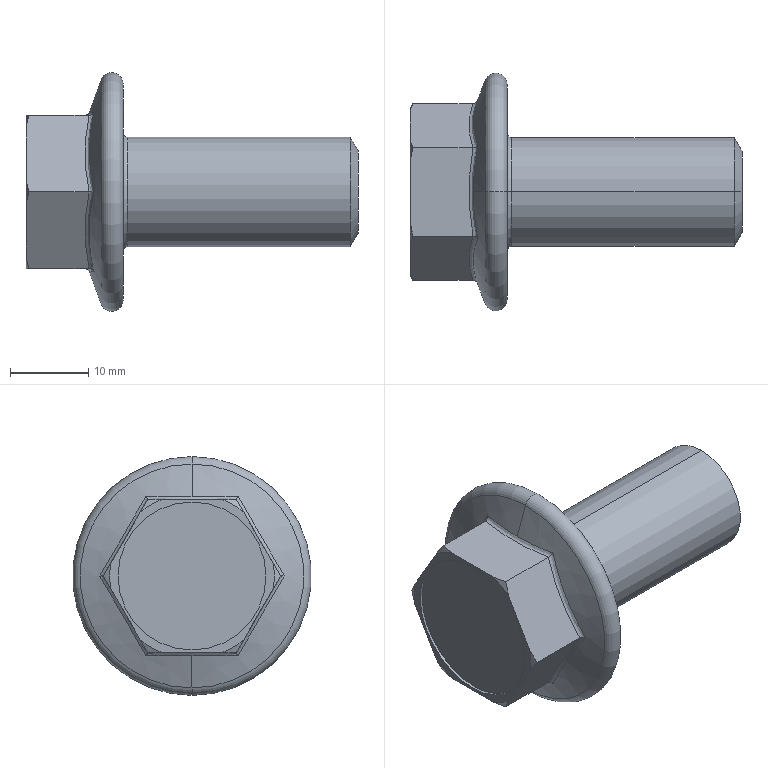Part | SolidWorks | features BaseBody 1 | 1 solid | 34 faces | box 42.4 x 30.5 x 30.5 mm | volume 9864 mm3 | plane 10 | cone 10 | spline 6 | torus 4 | cylinder 4 | commonest cylinder face diameters 14 x2 18.9 x2